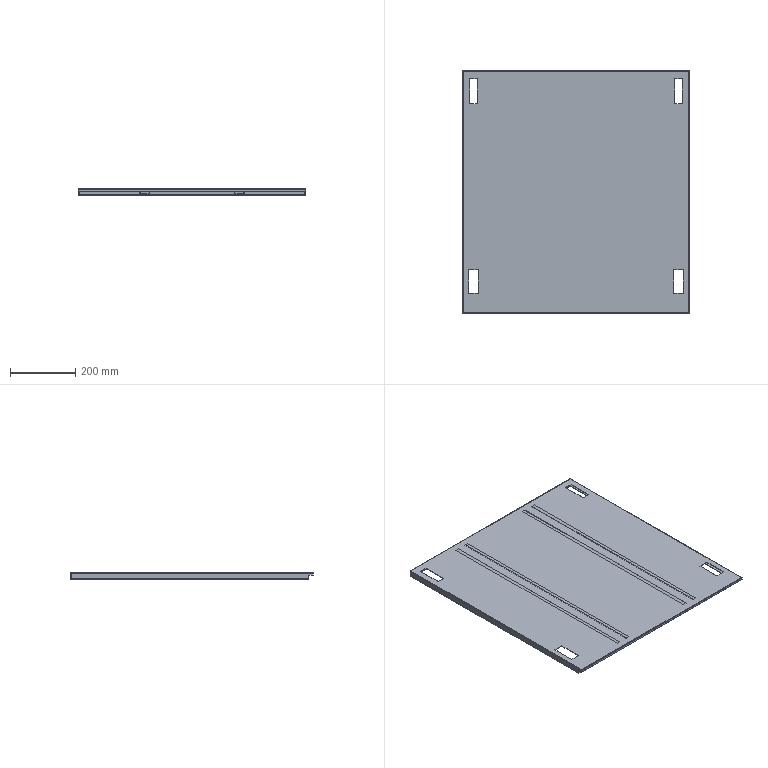Part | STEP file | FBDS-BJ-006 | 3 solids | 174 faces | box 696 x 746 x 20 mm | volume 1021844 mm3 | plane 132 | cylinder 30 | spline 12 | commonest cylinder face diameters 0.4 x15 3.4 x15